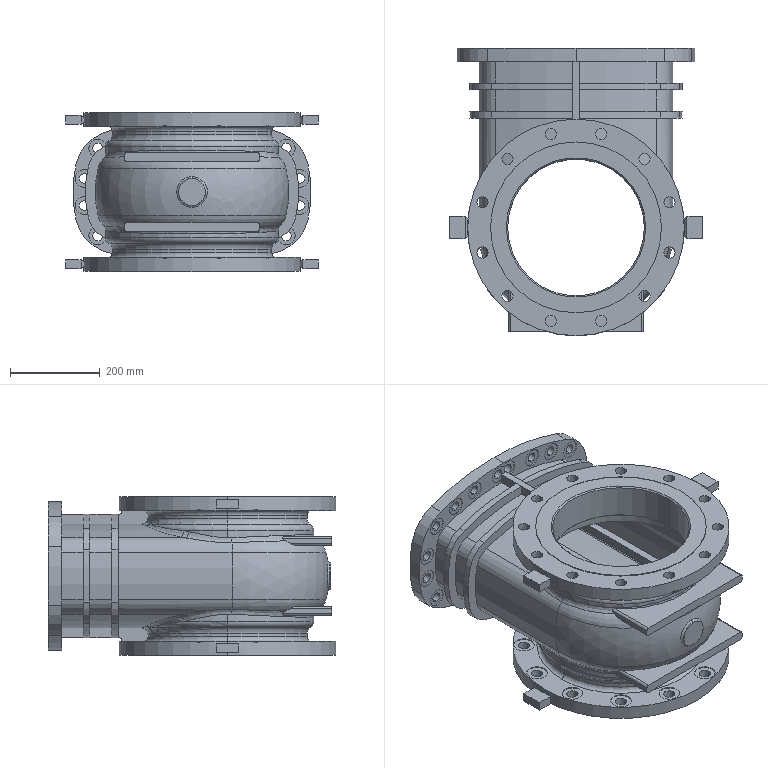Part | SolidWorks | features ICE 19, Fillet 7, MirrorPattern 4, MirrorSolid 4, Chamfer 3, CombineBodies 2, HoleWzd 2, Revolution 2, Split 2, Extrusion 1, MoveFace 1, RevCut 1, Rib 1, Sculpt 1 | 1 solid | 530 faces | box 563 x 641.5 x 356 mm | volume 21607642 mm3 | cylinder 304 | plane 152 | torus 28 | spline 26 | cone 18 | sphere 2 | commonest cylinder face diameters 25 x48 46 x48 40 x44 22 x40 10 x14 92 x12